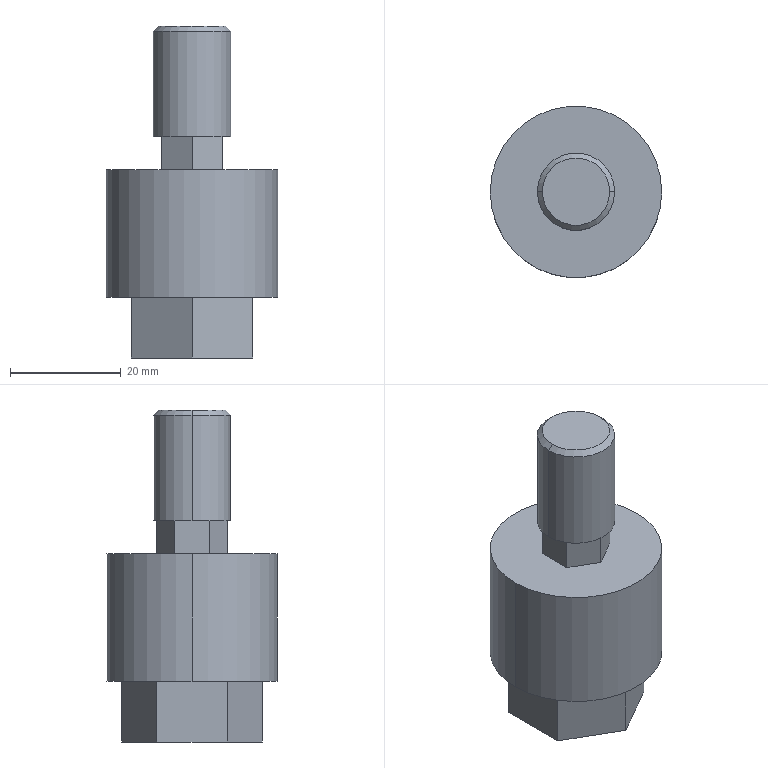Part | STEP file | JA40_14_150_JA40-14-150 | 1 solid | 28 faces | box 31 x 31 x 60 mm | volume 24083 mm3 | plane 18 | cylinder 6 | cone 4 | commonest cylinder face diameters 12.376 x2 14 x2 31 x2
STEP:
#1=CARTESIAN_POINT('',(-7.,0.,59.08));
#2=VERTEX_POINT('',#1);
#3=CARTESIAN_POINT('',(7.,0.,59.08));
#4=VERTEX_POINT('',#3);
#5=CARTESIAN_POINT('',(0.,0.,59.08));
#6=DIRECTION('',(0.,0.,-1.));
#7=DIRECTION('',(-1.,0.,0.));
#8=AXIS2_PLACEMENT_3D('',#5,#6,#7);
#9=CIRCLE('',#8,7.);
#10=EDGE_CURVE('',#2,#4,#9,.T.);
#11=ORIENTED_EDGE('',*,*,#10,.T.);
#12=CARTESIAN_POINT('',(7.,0.,40.));
#13=VERTEX_POINT('',#12);
#14=CARTESIAN_POINT('',(7.,0.,40.));
#15=DIRECTION('',(0.,0.,-1.));
#16=VECTOR('',#15,1000.);
#17=LINE('',#14,#16);
#18=EDGE_CURVE('',#4,#13,#17,.T.);
#19=ORIENTED_EDGE('',*,*,#18,.T.);
#20=CARTESIAN_POINT('',(-7.,0.,40.));
#21=VERTEX_POINT('',#20);
#22=CARTESIAN_POINT('',(0.,0.,40.));
#23=DIRECTION('',(0.,0.,-1.));
#24=DIRECTION('',(-1.,0.,0.));
#25=AXIS2_PLACEMENT_3D('',#22,#23,#24);
#26=CIRCLE('',#25,7.);
#27=EDGE_CURVE('',#21,#13,#26,.T.);
#28=ORIENTED_EDGE('',*,*,#27,.F.);
#29=CARTESIAN_POINT('',(-7.,0.,40.));
#30=DIRECTION('',(0.,0.,-1.));
#31=VECTOR('',#30,1000.);
#32=LINE('',#29,#31);
#33=EDGE_CURVE('',#2,#21,#32,.T.);
#34=ORIENTED_EDGE('',*,*,#33,.F.);
#35=EDGE_LOOP('',(#11,#19,#28,#34));
#36=FACE_OUTER_BOUND('',#35,.T.);
#37=CARTESIAN_POINT('',(0.,0.,40.));
#38=DIRECTION('',(0.,0.,-1.));
#39=DIRECTION('',(-1.,0.,0.));
#40=AXIS2_PLACEMENT_3D('',#37,#38,#39);
#41=CYLINDRICAL_SURFACE('',#40,7.);
#42=ADVANCED_FACE('',(#36),#41,.T.);
#43=CARTESIAN_POINT('',(-6.08,0.,60.));
#44=VERTEX_POINT('',#43);
#45=CARTESIAN_POINT('',(6.08,0.,60.));
#46=VERTEX_POINT('',#45);
#47=CARTESIAN_POINT('',(0.,0.,60.));
#48=DIRECTION('',(0.,0.,-1.));
#49=DIRECTION('',(-1.,0.,0.));
#50=AXIS2_PLACEMENT_3D('',#47,#48,#49);
#51=CIRCLE('',#50,6.08);
#52=EDGE_CURVE('',#44,#46,#51,.T.);
#53=ORIENTED_EDGE('',*,*,#52,.T.);
#54=CARTESIAN_POINT('',(7.,0.,59.08));
#55=DIRECTION('',(0.7071,0.,-0.7071));
#56=VECTOR('',#55,1000.);
#57=LINE('',#54,#56);
#58=EDGE_CURVE('',#46,#4,#57,.T.);
#59=ORIENTED_EDGE('',*,*,#58,.T.);
#60=ORIENTED_EDGE('',*,*,#10,.F.);
#61=CARTESIAN_POINT('',(-7.,0.,59.08));
#62=DIRECTION('',(-0.7071,0.,-0.7071));
#63=VECTOR('',#62,1000.);
#64=LINE('',#61,#63);
#65=EDGE_CURVE('',#44,#2,#64,.T.);
#66=ORIENTED_EDGE('',*,*,#65,.F.);
#67=EDGE_LOOP('',(#53,#59,#60,#66));
#68=FACE_OUTER_BOUND('',#67,.T.);
#69=CARTESIAN_POINT('',(0.,0.,59.08));
#70=DIRECTION('',(0.,0.,-1.));
#71=DIRECTION('',(-1.,0.,0.));
#72=AXIS2_PLACEMENT_3D('',#69,#70,#71);
#73=CONICAL_SURFACE('',#72,7.,0.7854);
#74=ADVANCED_FACE('',(#68),#73,.T.);
#75=CARTESIAN_POINT('',(6.188,0.,0.812));
#76=VERTEX_POINT('',#75);
#77=CARTESIAN_POINT('',(-6.188,0.,0.812));
#78=VERTEX_POINT('',#77);
#79=CARTESIAN_POINT('',(0.,0.,0.812));
#80=DIRECTION('',(0.,0.,-1.));
#81=DIRECTION('',(-1.,0.,0.));
#82=AXIS2_PLACEMENT_3D('',#79,#80,#81);
#83=CIRCLE('',#82,6.188);
#84=EDGE_CURVE('',#76,#78,#83,.T.);
#85=ORIENTED_EDGE('',*,*,#84,.F.);
#86=CARTESIAN_POINT('',(7.,0.,0.));
#87=VERTEX_POINT('',#86);
#88=CARTESIAN_POINT('',(6.188,0.,0.812));
#89=DIRECTION('',(0.7071,0.,-0.7071));
#90=VECTOR('',#89,1000.);
#91=LINE('',#88,#90);
#92=EDGE_CURVE('',#76,#87,#91,.T.);
#93=ORIENTED_EDGE('',*,*,#92,.T.);
#94=CARTESIAN_POINT('',(-7.,0.,0.));
#95=VERTEX_POINT('',#94);
#96=CARTESIAN_POINT('',(0.,0.,0.));
#97=DIRECTION('',(0.,0.,-1.));
#98=DIRECTION('',(-1.,0.,0.));
#99=AXIS2_PLACEMENT_3D('',#96,#97,#98);
#100=CIRCLE('',#99,7.);
#101=EDGE_CURVE('',#87,#95,#100,.T.);
#102=ORIENTED_EDGE('',*,*,#101,.T.);
#103=CARTESIAN_POINT('',(-6.188,0.,0.812));
#104=DIRECTION('',(-0.7071,0.,-0.7071));
#105=VECTOR('',#104,1000.);
#106=LINE('',#103,#105);
#107=EDGE_CURVE('',#78,#95,#106,.T.);
#108=ORIENTED_EDGE('',*,*,#107,.F.);
#109=EDGE_LOOP('',(#85,#93,#102,#108));
#110=FACE_OUTER_BOUND('',#109,.T.);
#111=CARTESIAN_POINT('',(0.,0.,0.812));
#112=DIRECTION('',(0.,0.,-1.));
#113=DIRECTION('',(-1.,0.,0.));
#114=AXIS2_PLACEMENT_3D('',#111,#112,#113);
#115=CONICAL_SURFACE('',#114,6.188,0.7854);
#116=ADVANCED_FACE('',(#110),#115,.F.);
#117=CARTESIAN_POINT('',(6.188,0.,13.));
#118=VERTEX_POINT('',#117);
#119=CARTESIAN_POINT('',(-6.188,0.,13.));
#120=VERTEX_POINT('',#119);
#121=CARTESIAN_POINT('',(0.,0.,13.));
#122=DIRECTION('',(0.,0.,-1.));
#123=DIRECTION('',(-1.,0.,0.));
#124=AXIS2_PLACEMENT_3D('',#121,#122,#123);
#125=CIRCLE('',#124,6.188);
#126=EDGE_CURVE('',#118,#120,#125,.T.);
#127=ORIENTED_EDGE('',*,*,#126,.F.);
#128=CARTESIAN_POINT('',(6.188,0.,0.));
#129=DIRECTION('',(0.,0.,-1.));
#130=VECTOR('',#129,1000.);
#131=LINE('',#128,#130);
#132=EDGE_CURVE('',#118,#76,#131,.T.);
#133=ORIENTED_EDGE('',*,*,#132,.T.);
#134=ORIENTED_EDGE('',*,*,#84,.T.);
#135=CARTESIAN_POINT('',(-6.188,0.,0.));
#136=DIRECTION('',(0.,0.,-1.));
#137=VECTOR('',#136,1000.);
#138=LINE('',#135,#137);
#139=EDGE_CURVE('',#120,#78,#138,.T.);
#140=ORIENTED_EDGE('',*,*,#139,.F.);
#141=EDGE_LOOP('',(#127,#133,#134,#140));
#142=FACE_OUTER_BOUND('',#141,.T.);
#143=CARTESIAN_POINT('',(0.,0.,0.));
#144=DIRECTION('',(0.,0.,-1.));
#145=DIRECTION('',(-1.,0.,0.));
#146=AXIS2_PLACEMENT_3D('',#143,#144,#145);
#147=CYLINDRICAL_SURFACE('',#146,6.188);
#148=ADVANCED_FACE('',(#142),#147,.F.);
#149=CARTESIAN_POINT('',(-15.5,0.,34.));
#150=VERTEX_POINT('',#149);
#151=CARTESIAN_POINT('',(15.5,0.,34.));
#152=VERTEX_POINT('',#151);
#153=CARTESIAN_POINT('',(0.,0.,34.));
#154=DIRECTION('',(0.,0.,-1.));
#155=DIRECTION('',(-1.,0.,0.));
#156=AXIS2_PLACEMENT_3D('',#153,#154,#155);
#157=CIRCLE('',#156,15.5);
#158=EDGE_CURVE('',#150,#152,#157,.T.);
#159=ORIENTED_EDGE('',*,*,#158,.T.);
#160=CARTESIAN_POINT('',(15.5,0.,11.));
#161=VERTEX_POINT('',#160);
#162=CARTESIAN_POINT('',(15.5,0.,0.));
#163=DIRECTION('',(0.,0.,-1.));
#164=VECTOR('',#163,1000.);
#165=LINE('',#162,#164);
#166=EDGE_CURVE('',#152,#161,#165,.T.);
#167=ORIENTED_EDGE('',*,*,#166,.T.);
#168=CARTESIAN_POINT('',(-15.5,0.,11.));
#169=VERTEX_POINT('',#168);
#170=CARTESIAN_POINT('',(0.,0.,11.));
#171=DIRECTION('',(0.,0.,-1.));
#172=DIRECTION('',(-1.,0.,0.));
#173=AXIS2_PLACEMENT_3D('',#170,#171,#172);
#174=CIRCLE('',#173,15.5);
#175=EDGE_CURVE('',#169,#161,#174,.T.);
#176=ORIENTED_EDGE('',*,*,#175,.F.);
#177=CARTESIAN_POINT('',(-15.5,0.,0.));
#178=DIRECTION('',(0.,0.,-1.));
#179=VECTOR('',#178,1000.);
#180=LINE('',#177,#179);
#181=EDGE_CURVE('',#150,#169,#180,.T.);
#182=ORIENTED_EDGE('',*,*,#181,.F.);
#183=EDGE_LOOP('',(#159,#167,#176,#182));
#184=FACE_OUTER_BOUND('',#183,.T.);
#185=CARTESIAN_POINT('',(0.,0.,0.));
#186=DIRECTION('',(0.,0.,-1.));
#187=DIRECTION('',(-1.,0.,0.));
#188=AXIS2_PLACEMENT_3D('',#185,#186,#187);
#189=CYLINDRICAL_SURFACE('',#188,15.5);
#190=ADVANCED_FACE('',(#184),#189,.T.);
#191=CARTESIAN_POINT('',(0.,6.351,40.));
#192=VERTEX_POINT('',#191);
#193=CARTESIAN_POINT('',(-5.5,3.175,40.));
#194=VERTEX_POINT('',#193);
#195=CARTESIAN_POINT('',(0.,6.351,40.));
#196=DIRECTION('',(-0.866,-0.5,0.));
#197=VECTOR('',#196,1000.);
#198=LINE('',#195,#197);
#199=EDGE_CURVE('',#192,#194,#198,.T.);
#200=ORIENTED_EDGE('',*,*,#199,.F.);
#201=CARTESIAN_POINT('',(0.,6.351,34.));
#202=VERTEX_POINT('',#201);
#203=CARTESIAN_POINT('',(0.,6.351,34.));
#204=DIRECTION('',(0.,0.,1.));
#205=VECTOR('',#204,1000.);
#206=LINE('',#203,#205);
#207=EDGE_CURVE('',#202,#192,#206,.T.);
#208=ORIENTED_EDGE('',*,*,#207,.F.);
#209=CARTESIAN_POINT('',(-5.5,3.175,34.));
#210=VERTEX_POINT('',#209);
#211=CARTESIAN_POINT('',(0.,6.351,34.));
#212=DIRECTION('',(-0.866,-0.5,0.));
#213=VECTOR('',#212,1000.);
#214=LINE('',#211,#213);
#215=EDGE_CURVE('',#202,#210,#214,.T.);
#216=ORIENTED_EDGE('',*,*,#215,.T.);
#217=CARTESIAN_POINT('',(-5.5,3.175,34.));
#218=DIRECTION('',(0.,0.,1.));
#219=VECTOR('',#218,1000.);
#220=LINE('',#217,#219);
#221=EDGE_CURVE('',#210,#194,#220,.T.);
#222=ORIENTED_EDGE('',*,*,#221,.T.);
#223=EDGE_LOOP('',(#200,#208,#216,#222));
#224=FACE_OUTER_BOUND('',#223,.T.);
#225=CARTESIAN_POINT('',(0.,6.351,34.));
#226=DIRECTION('',(-0.5,0.866,0.));
#227=DIRECTION('',(-0.866,-0.5,0.));
#228=AXIS2_PLACEMENT_3D('',#225,#226,#227);
#229=PLANE('',#228);
#230=ADVANCED_FACE('',(#224),#229,.T.);
#231=CARTESIAN_POINT('',(5.5,3.175,40.));
#232=VERTEX_POINT('',#231);
#233=CARTESIAN_POINT('',(5.5,3.175,40.));
#234=DIRECTION('',(-0.866,0.5,0.));
#235=VECTOR('',#234,1000.);
#236=LINE('',#233,#235);
#237=EDGE_CURVE('',#232,#192,#236,.T.);
#238=ORIENTED_EDGE('',*,*,#237,.F.);
#239=CARTESIAN_POINT('',(5.5,3.175,34.));
#240=VERTEX_POINT('',#239);
#241=CARTESIAN_POINT('',(5.5,3.175,34.));
#242=DIRECTION('',(0.,0.,1.));
#243=VECTOR('',#242,1000.);
#244=LINE('',#241,#243);
#245=EDGE_CURVE('',#240,#232,#244,.T.);
#246=ORIENTED_EDGE('',*,*,#245,.F.);
#247=CARTESIAN_POINT('',(5.5,3.175,34.));
#248=DIRECTION('',(-0.866,0.5,0.));
#249=VECTOR('',#248,1000.);
#250=LINE('',#247,#249);
#251=EDGE_CURVE('',#240,#202,#250,.T.);
#252=ORIENTED_EDGE('',*,*,#251,.T.);
#253=ORIENTED_EDGE('',*,*,#207,.T.);
#254=EDGE_LOOP('',(#238,#246,#252,#253));
#255=FACE_OUTER_BOUND('',#254,.T.);
#256=CARTESIAN_POINT('',(5.5,3.175,34.));
#257=DIRECTION('',(0.5,0.866,0.));
#258=DIRECTION('',(-0.866,0.5,0.));
#259=AXIS2_PLACEMENT_3D('',#256,#257,#258);
#260=PLANE('',#259);
#261=ADVANCED_FACE('',(#255),#260,.T.);
#262=CARTESIAN_POINT('',(5.5,-3.175,40.));
#263=VERTEX_POINT('',#262);
#264=CARTESIAN_POINT('',(5.5,-3.175,40.));
#265=DIRECTION('',(0.,1.,0.));
#266=VECTOR('',#265,1000.);
#267=LINE('',#264,#266);
#268=EDGE_CURVE('',#263,#232,#267,.T.);
#269=ORIENTED_EDGE('',*,*,#268,.F.);
#270=CARTESIAN_POINT('',(5.5,-3.175,34.));
#271=VERTEX_POINT('',#270);
#272=CARTESIAN_POINT('',(5.5,-3.175,34.));
#273=DIRECTION('',(0.,0.,1.));
#274=VECTOR('',#273,1000.);
#275=LINE('',#272,#274);
#276=EDGE_CURVE('',#271,#263,#275,.T.);
#277=ORIENTED_EDGE('',*,*,#276,.F.);
#278=CARTESIAN_POINT('',(5.5,-3.175,34.));
#279=DIRECTION('',(0.,1.,0.));
#280=VECTOR('',#279,1000.);
#281=LINE('',#278,#280);
#282=EDGE_CURVE('',#271,#240,#281,.T.);
#283=ORIENTED_EDGE('',*,*,#282,.T.);
#284=ORIENTED_EDGE('',*,*,#245,.T.);
#285=EDGE_LOOP('',(#269,#277,#283,#284));
#286=FACE_OUTER_BOUND('',#285,.T.);
#287=CARTESIAN_POINT('',(5.5,-3.175,34.));
#288=DIRECTION('',(1.,0.,0.));
#289=DIRECTION('',(0.,0.,-1.));
#290=AXIS2_PLACEMENT_3D('',#287,#288,#289);
#291=PLANE('',#290);
#292=ADVANCED_FACE('',(#286),#291,.T.);
#293=CARTESIAN_POINT('',(0.,-6.351,40.));
#294=VERTEX_POINT('',#293);
#295=CARTESIAN_POINT('',(0.,-6.351,40.));
#296=DIRECTION('',(0.866,0.5,0.));
#297=VECTOR('',#296,1000.);
#298=LINE('',#295,#297);
#299=EDGE_CURVE('',#294,#263,#298,.T.);
#300=ORIENTED_EDGE('',*,*,#299,.F.);
#301=CARTESIAN_POINT('',(0.,-6.351,34.));
#302=VERTEX_POINT('',#301);
#303=CARTESIAN_POINT('',(0.,-6.351,34.));
#304=DIRECTION('',(0.,0.,1.));
#305=VECTOR('',#304,1000.);
#306=LINE('',#303,#305);
#307=EDGE_CURVE('',#302,#294,#306,.T.);
#308=ORIENTED_EDGE('',*,*,#307,.F.);
#309=CARTESIAN_POINT('',(0.,-6.351,34.));
#310=DIRECTION('',(0.866,0.5,0.));
#311=VECTOR('',#310,1000.);
#312=LINE('',#309,#311);
#313=EDGE_CURVE('',#302,#271,#312,.T.);
#314=ORIENTED_EDGE('',*,*,#313,.T.);
#315=ORIENTED_EDGE('',*,*,#276,.T.);
#316=EDGE_LOOP('',(#300,#308,#314,#315));
#317=FACE_OUTER_BOUND('',#316,.T.);
#318=CARTESIAN_POINT('',(0.,-6.351,34.));
#319=DIRECTION('',(0.5,-0.866,0.));
#320=DIRECTION('',(0.866,0.5,0.));
#321=AXIS2_PLACEMENT_3D('',#318,#319,#320);
#322=PLANE('',#321);
#323=ADVANCED_FACE('',(#317),#322,.T.);
#324=CARTESIAN_POINT('',(-5.5,-3.175,40.));
#325=VERTEX_POINT('',#324);
#326=CARTESIAN_POINT('',(-5.5,-3.175,40.));
#327=DIRECTION('',(0.866,-0.5,0.));
#328=VECTOR('',#327,1000.);
#329=LINE('',#326,#328);
#330=EDGE_CURVE('',#325,#294,#329,.T.);
#331=ORIENTED_EDGE('',*,*,#330,.F.);
#332=CARTESIAN_POINT('',(-5.5,-3.175,34.));
#333=VERTEX_POINT('',#332);
#334=CARTESIAN_POINT('',(-5.5,-3.175,34.));
#335=DIRECTION('',(0.,0.,1.));
#336=VECTOR('',#335,1000.);
#337=LINE('',#334,#336);
#338=EDGE_CURVE('',#333,#325,#337,.T.);
#339=ORIENTED_EDGE('',*,*,#338,.F.);
#340=CARTESIAN_POINT('',(-5.5,-3.175,34.));
#341=DIRECTION('',(0.866,-0.5,0.));
#342=VECTOR('',#341,1000.);
#343=LINE('',#340,#342);
#344=EDGE_CURVE('',#333,#302,#343,.T.);
#345=ORIENTED_EDGE('',*,*,#344,.T.);
#346=ORIENTED_EDGE('',*,*,#307,.T.);
#347=EDGE_LOOP('',(#331,#339,#345,#346));
#348=FACE_OUTER_BOUND('',#347,.T.);
#349=CARTESIAN_POINT('',(-5.5,-3.175,34.));
#350=DIRECTION('',(-0.5,-0.866,0.));
#351=DIRECTION('',(0.866,-0.5,0.));
#352=AXIS2_PLACEMENT_3D('',#349,#350,#351);
#353=PLANE('',#352);
#354=ADVANCED_FACE('',(#348),#353,.T.);
#355=CARTESIAN_POINT('',(-5.5,3.175,40.));
#356=DIRECTION('',(0.,-1.,0.));
#357=VECTOR('',#356,1000.);
#358=LINE('',#355,#357);
#359=EDGE_CURVE('',#194,#325,#358,.T.);
#360=ORIENTED_EDGE('',*,*,#359,.F.);
#361=ORIENTED_EDGE('',*,*,#221,.F.);
#362=CARTESIAN_POINT('',(-5.5,3.175,34.));
#363=DIRECTION('',(0.,-1.,0.));
#364=VECTOR('',#363,1000.);
#365=LINE('',#362,#364);
#366=EDGE_CURVE('',#210,#333,#365,.T.);
#367=ORIENTED_EDGE('',*,*,#366,.T.);
#368=ORIENTED_EDGE('',*,*,#338,.T.);
#369=EDGE_LOOP('',(#360,#361,#367,#368));
#370=FACE_OUTER_BOUND('',#369,.T.);
#371=CARTESIAN_POINT('',(-5.5,3.175,34.));
#372=DIRECTION('',(-1.,0.,0.));
#373=DIRECTION('',(0.,0.,1.));
#374=AXIS2_PLACEMENT_3D('',#371,#372,#373);
#375=PLANE('',#374);
#376=ADVANCED_FACE('',(#370),#375,.T.);
#377=ORIENTED_EDGE('',*,*,#366,.F.);
#378=ORIENTED_EDGE('',*,*,#215,.F.);
#379=ORIENTED_EDGE('',*,*,#251,.F.);
#380=ORIENTED_EDGE('',*,*,#282,.F.);
#381=ORIENTED_EDGE('',*,*,#313,.F.);
#382=ORIENTED_EDGE('',*,*,#344,.F.);
#383=EDGE_LOOP('',(#377,#378,#379,#380,#381,#382));
#384=FACE_BOUND('',#383,.T.);
#385=ORIENTED_EDGE('',*,*,#158,.F.);
#386=CARTESIAN_POINT('',(0.,0.,34.));
#387=DIRECTION('',(0.,0.,-1.));
#388=DIRECTION('',(-1.,0.,0.));
#389=AXIS2_PLACEMENT_3D('',#386,#387,#388);
#390=CIRCLE('',#389,15.5);
#391=EDGE_CURVE('',#152,#150,#390,.T.);
#392=ORIENTED_EDGE('',*,*,#391,.F.);
#393=EDGE_LOOP('',(#385,#392));
#394=FACE_OUTER_BOUND('',#393,.T.);
#395=CARTESIAN_POINT('',(0.,0.,34.));
#396=DIRECTION('',(0.,0.,1.));
#397=DIRECTION('',(1.,0.,0.));
#398=AXIS2_PLACEMENT_3D('',#395,#396,#397);
#399=PLANE('',#398);
#400=ADVANCED_FACE('',(#384,#394),#399,.T.);
#401=ORIENTED_EDGE('',*,*,#166,.F.);
#402=ORIENTED_EDGE('',*,*,#391,.T.);
#403=ORIENTED_EDGE('',*,*,#181,.T.);
#404=CARTESIAN_POINT('',(0.,0.,11.));
#405=DIRECTION('',(0.,0.,-1.));
#406=DIRECTION('',(-1.,0.,0.));
#407=AXIS2_PLACEMENT_3D('',#404,#405,#406);
#408=CIRCLE('',#407,15.5);
#409=EDGE_CURVE('',#161,#169,#408,.T.);
#410=ORIENTED_EDGE('',*,*,#409,.F.);
#411=EDGE_LOOP('',(#401,#402,#403,#410));
#412=FACE_OUTER_BOUND('',#411,.T.);
#413=CARTESIAN_POINT('',(0.,0.,0.));
#414=DIRECTION('',(0.,0.,-1.));
#415=DIRECTION('',(-1.,0.,0.));
#416=AXIS2_PLACEMENT_3D('',#413,#414,#415);
#417=CYLINDRICAL_SURFACE('',#416,15.5);
#418=ADVANCED_FACE('',(#412),#417,.T.);
#419=ORIENTED_EDGE('',*,*,#175,.T.);
#420=ORIENTED_EDGE('',*,*,#409,.T.);
#421=EDGE_LOOP('',(#419,#420));
#422=FACE_OUTER_BOUND('',#421,.T.);
#423=CARTESIAN_POINT('',(-11.,6.351,11.));
#424=VERTEX_POINT('',#423);
#425=CARTESIAN_POINT('',(-11.,-6.351,11.));
#426=VERTEX_POINT('',#425);
#427=CARTESIAN_POINT('',(-11.,6.351,11.));
#428=DIRECTION('',(0.,-1.,0.));
#429=VECTOR('',#428,1000.);
#430=LINE('',#427,#429);
#431=EDGE_CURVE('',#424,#426,#430,.T.);
#432=ORIENTED_EDGE('',*,*,#431,.T.);
#433=CARTESIAN_POINT('',(0.,-12.702,11.));
#434=VERTEX_POINT('',#433);
#435=CARTESIAN_POINT('',(-11.,-6.351,11.));
#436=DIRECTION('',(0.866,-0.5,0.));
#437=VECTOR('',#436,1000.);
#438=LINE('',#435,#437);
#439=EDGE_CURVE('',#426,#434,#438,.T.);
#440=ORIENTED_EDGE('',*,*,#439,.T.);
#441=CARTESIAN_POINT('',(11.,-6.351,11.));
#442=VERTEX_POINT('',#441);
#443=CARTESIAN_POINT('',(0.,-12.702,11.));
#444=DIRECTION('',(0.866,0.5,0.));
#445=VECTOR('',#444,1000.);
#446=LINE('',#443,#445);
#447=EDGE_CURVE('',#434,#442,#446,.T.);
#448=ORIENTED_EDGE('',*,*,#447,.T.);
#449=CARTESIAN_POINT('',(11.,6.351,11.));
#450=VERTEX_POINT('',#449);
#451=CARTESIAN_POINT('',(11.,-6.351,11.));
#452=DIRECTION('',(0.,1.,0.));
#453=VECTOR('',#452,1000.);
#454=LINE('',#451,#453);
#455=EDGE_CURVE('',#442,#450,#454,.T.);
#456=ORIENTED_EDGE('',*,*,#455,.T.);
#457=CARTESIAN_POINT('',(0.,12.702,11.));
#458=VERTEX_POINT('',#457);
#459=CARTESIAN_POINT('',(11.,6.351,11.));
#460=DIRECTION('',(-0.866,0.5,0.));
#461=VECTOR('',#460,1000.);
#462=LINE('',#459,#461);
#463=EDGE_CURVE('',#450,#458,#462,.T.);
#464=ORIENTED_EDGE('',*,*,#463,.T.);
#465=CARTESIAN_POINT('',(0.,12.702,11.));
#466=DIRECTION('',(-0.866,-0.5,0.));
#467=VECTOR('',#466,1000.);
#468=LINE('',#465,#467);
#469=EDGE_CURVE('',#458,#424,#468,.T.);
#470=ORIENTED_EDGE('',*,*,#469,.T.);
#471=EDGE_LOOP('',(#432,#440,#448,#456,#464,#470));
#472=FACE_BOUND('',#471,.T.);
#473=CARTESIAN_POINT('',(0.,15.5,11.));
#474=DIRECTION('',(0.,0.,-1.));
#475=DIRECTION('',(-1.,0.,0.));
#476=AXIS2_PLACEMENT_3D('',#473,#474,#475);
#477=PLANE('',#476);
#478=ADVANCED_FACE('',(#422,#472),#477,.T.);
#479=CARTESIAN_POINT('',(0.,12.702,0.));
#480=VERTEX_POINT('',#479);
#481=CARTESIAN_POINT('',(-11.,6.351,0.));
#482=VERTEX_POINT('',#481);
#483=CARTESIAN_POINT('',(0.,12.702,0.));
#484=DIRECTION('',(-0.866,-0.5,0.));
#485=VECTOR('',#484,1000.);
#486=LINE('',#483,#485);
#487=EDGE_CURVE('',#480,#482,#486,.T.);
#488=ORIENTED_EDGE('',*,*,#487,.T.);
#489=CARTESIAN_POINT('',(-11.,6.351,11.));
#490=DIRECTION('',(0.,0.,-1.));
#491=VECTOR('',#490,1000.);
#492=LINE('',#489,#491);
#493=EDGE_CURVE('',#424,#482,#492,.T.);
#494=ORIENTED_EDGE('',*,*,#493,.F.);
#495=ORIENTED_EDGE('',*,*,#469,.F.);
#496=CARTESIAN_POINT('',(0.,12.702,11.));
#497=DIRECTION('',(0.,0.,-1.));
#498=VECTOR('',#497,1000.);
#499=LINE('',#496,#498);
#500=EDGE_CURVE('',#458,#480,#499,.T.);
#501=ORIENTED_EDGE('',*,*,#500,.T.);
#502=EDGE_LOOP('',(#488,#494,#495,#501));
#503=FACE_OUTER_BOUND('',#502,.T.);
#504=CARTESIAN_POINT('',(0.,12.702,11.));
#505=DIRECTION('',(0.5,-0.866,0.));
#506=DIRECTION('',(0.866,0.5,0.));
#507=AXIS2_PLACEMENT_3D('',#504,#505,#506);
#508=PLANE('',#507);
#509=ADVANCED_FACE('',(#503),#508,.F.);
#510=CARTESIAN_POINT('',(-11.,-6.351,0.));
#511=VERTEX_POINT('',#510);
#512=CARTESIAN_POINT('',(-11.,6.351,0.));
#513=DIRECTION('',(0.,-1.,0.));
#514=VECTOR('',#513,1000.);
#515=LINE('',#512,#514);
#516=EDGE_CURVE('',#482,#511,#515,.T.);
#517=ORIENTED_EDGE('',*,*,#516,.T.);
#518=CARTESIAN_POINT('',(-11.,-6.351,11.));
#519=DIRECTION('',(0.,0.,-1.));
#520=VECTOR('',#519,1000.);
#521=LINE('',#518,#520);
#522=EDGE_CURVE('',#426,#511,#521,.T.);
#523=ORIENTED_EDGE('',*,*,#522,.F.);
#524=ORIENTED_EDGE('',*,*,#431,.F.);
#525=ORIENTED_EDGE('',*,*,#493,.T.);
#526=EDGE_LOOP('',(#517,#523,#524,#525));
#527=FACE_OUTER_BOUND('',#526,.T.);
#528=CARTESIAN_POINT('',(-11.,6.351,11.));
#529=DIRECTION('',(1.,0.,0.));
#530=DIRECTION('',(0.,0.,-1.));
#531=AXIS2_PLACEMENT_3D('',#528,#529,#530);
#532=PLANE('',#531);
#533=ADVANCED_FACE('',(#527),#532,.F.);
#534=CARTESIAN_POINT('',(0.,-12.702,0.));
#535=VERTEX_POINT('',#534);
#536=CARTESIAN_POINT('',(-11.,-6.351,0.));
#537=DIRECTION('',(0.866,-0.5,0.));
#538=VECTOR('',#537,1000.);
#539=LINE('',#536,#538);
#540=EDGE_CURVE('',#511,#535,#539,.T.);
#541=ORIENTED_EDGE('',*,*,#540,.T.);
#542=CARTESIAN_POINT('',(0.,-12.702,11.));
#543=DIRECTION('',(0.,0.,-1.));
#544=VECTOR('',#543,1000.);
#545=LINE('',#542,#544);
#546=EDGE_CURVE('',#434,#535,#545,.T.);
#547=ORIENTED_EDGE('',*,*,#546,.F.);
#548=ORIENTED_EDGE('',*,*,#439,.F.);
#549=ORIENTED_EDGE('',*,*,#522,.T.);
#550=EDGE_LOOP('',(#541,#547,#548,#549));
#551=FACE_OUTER_BOUND('',#550,.T.);
#552=CARTESIAN_POINT('',(-11.,-6.351,11.));
#553=DIRECTION('',(0.5,0.866,0.));
#554=DIRECTION('',(-0.866,0.5,0.));
#555=AXIS2_PLACEMENT_3D('',#552,#553,#554);
#556=PLANE('',#555);
#557=ADVANCED_FACE('',(#551),#556,.F.);
#558=CARTESIAN_POINT('',(11.,-6.351,0.));
#559=VERTEX_POINT('',#558);
#560=CARTESIAN_POINT('',(0.,-12.702,0.));
#561=DIRECTION('',(0.866,0.5,0.));
#562=VECTOR('',#561,1000.);
#563=LINE('',#560,#562);
#564=EDGE_CURVE('',#535,#559,#563,.T.);
#565=ORIENTED_EDGE('',*,*,#564,.T.);
#566=CARTESIAN_POINT('',(11.,-6.351,11.));
#567=DIRECTION('',(0.,0.,-1.));
#568=VECTOR('',#567,1000.);
#569=LINE('',#566,#568);
#570=EDGE_CURVE('',#442,#559,#569,.T.);
#571=ORIENTED_EDGE('',*,*,#570,.F.);
#572=ORIENTED_EDGE('',*,*,#447,.F.);
#573=ORIENTED_EDGE('',*,*,#546,.T.);
#574=EDGE_LOOP('',(#565,#571,#572,#573));
#575=FACE_OUTER_BOUND('',#574,.T.);
#576=CARTESIAN_POINT('',(0.,-12.702,11.));
#577=DIRECTION('',(-0.5,0.866,0.));
#578=DIRECTION('',(-0.866,-0.5,0.));
#579=AXIS2_PLACEMENT_3D('',#576,#577,#578);
#580=PLANE('',#579);
#581=ADVANCED_FACE('',(#575),#580,.F.);
#582=CARTESIAN_POINT('',(11.,6.351,0.));
#583=VERTEX_POINT('',#582);
#584=CARTESIAN_POINT('',(11.,-6.351,0.));
#585=DIRECTION('',(0.,1.,0.));
#586=VECTOR('',#585,1000.);
#587=LINE('',#584,#586);
#588=EDGE_CURVE('',#559,#583,#587,.T.);
#589=ORIENTED_EDGE('',*,*,#588,.T.);
#590=CARTESIAN_POINT('',(11.,6.351,11.));
#591=DIRECTION('',(0.,0.,-1.));
#592=VECTOR('',#591,1000.);
#593=LINE('',#590,#592);
#594=EDGE_CURVE('',#450,#583,#593,.T.);
#595=ORIENTED_EDGE('',*,*,#594,.F.);
#596=ORIENTED_EDGE('',*,*,#455,.F.);
#597=ORIENTED_EDGE('',*,*,#570,.T.);
#598=EDGE_LOOP('',(#589,#595,#596,#597));
#599=FACE_OUTER_BOUND('',#598,.T.);
#600=CARTESIAN_POINT('',(11.,-6.351,11.));
#601=DIRECTION('',(-1.,0.,0.));
#602=DIRECTION('',(0.,0.,1.));
#603=AXIS2_PLACEMENT_3D('',#600,#601,#602);
#604=PLANE('',#603);
#605=ADVANCED_FACE('',(#599),#604,.F.);
#606=CARTESIAN_POINT('',(11.,6.351,0.));
#607=DIRECTION('',(-0.866,0.5,0.));
#608=VECTOR('',#607,1000.);
#609=LINE('',#606,#608);
#610=EDGE_CURVE('',#583,#480,#609,.T.);
#611=ORIENTED_EDGE('',*,*,#610,.T.);
#612=ORIENTED_EDGE('',*,*,#500,.F.);
#613=ORIENTED_EDGE('',*,*,#463,.F.);
#614=ORIENTED_EDGE('',*,*,#594,.T.);
#615=EDGE_LOOP('',(#611,#612,#613,#614));
#616=FACE_OUTER_BOUND('',#615,.T.);
#617=CARTESIAN_POINT('',(11.,6.351,11.));
#618=DIRECTION('',(-0.5,-0.866,0.));
#619=DIRECTION('',(0.866,-0.5,0.));
#620=AXIS2_PLACEMENT_3D('',#617,#618,#619);
#621=PLANE('',#620);
#622=ADVANCED_FACE('',(#616),#621,.F.);
#623=CARTESIAN_POINT('',(0.,0.,13.));
#624=DIRECTION('',(0.,0.,-1.));
#625=DIRECTION('',(-1.,0.,0.));
#626=AXIS2_PLACEMENT_3D('',#623,#624,#625);
#627=CIRCLE('',#626,6.188);
#628=EDGE_CURVE('',#120,#118,#627,.T.);
#629=ORIENTED_EDGE('',*,*,#628,.T.);
#630=ORIENTED_EDGE('',*,*,#126,.T.);
#631=EDGE_LOOP('',(#629,#630));
#632=FACE_OUTER_BOUND('',#631,.T.);
#633=CARTESIAN_POINT('',(0.,6.188,13.));
#634=DIRECTION('',(0.,0.,-1.));
#635=DIRECTION('',(-1.,0.,0.));
#636=AXIS2_PLACEMENT_3D('',#633,#634,#635);
#637=PLANE('',#636);
#638=ADVANCED_FACE('',(#632),#637,.T.);
#639=ORIENTED_EDGE('',*,*,#132,.F.);
#640=ORIENTED_EDGE('',*,*,#628,.F.);
#641=ORIENTED_EDGE('',*,*,#139,.T.);
#642=CARTESIAN_POINT('',(0.,0.,0.812));
#643=DIRECTION('',(0.,0.,-1.));
#644=DIRECTION('',(-1.,0.,0.));
#645=AXIS2_PLACEMENT_3D('',#642,#643,#644);
#646=CIRCLE('',#645,6.188);
#647=EDGE_CURVE('',#78,#76,#646,.T.);
#648=ORIENTED_EDGE('',*,*,#647,.T.);
#649=EDGE_LOOP('',(#639,#640,#641,#648));
#650=FACE_OUTER_BOUND('',#649,.T.);
#651=CARTESIAN_POINT('',(0.,0.,0.));
#652=DIRECTION('',(0.,0.,-1.));
#653=DIRECTION('',(-1.,0.,0.));
#654=AXIS2_PLACEMENT_3D('',#651,#652,#653);
#655=CYLINDRICAL_SURFACE('',#654,6.188);
#656=ADVANCED_FACE('',(#650),#655,.F.);
#657=ORIENTED_EDGE('',*,*,#92,.F.);
#658=ORIENTED_EDGE('',*,*,#647,.F.);
#659=ORIENTED_EDGE('',*,*,#107,.T.);
#660=CARTESIAN_POINT('',(0.,0.,0.));
#661=DIRECTION('',(0.,0.,-1.));
#662=DIRECTION('',(-1.,0.,0.));
#663=AXIS2_PLACEMENT_3D('',#660,#661,#662);
#664=CIRCLE('',#663,7.);
#665=EDGE_CURVE('',#95,#87,#664,.T.);
#666=ORIENTED_EDGE('',*,*,#665,.T.);
#667=EDGE_LOOP('',(#657,#658,#659,#666));
#668=FACE_OUTER_BOUND('',#667,.T.);
#669=CARTESIAN_POINT('',(0.,0.,0.812));
#670=DIRECTION('',(0.,0.,-1.));
#671=DIRECTION('',(-1.,0.,0.));
#672=AXIS2_PLACEMENT_3D('',#669,#670,#671);
#673=CONICAL_SURFACE('',#672,6.188,0.7854);
#674=ADVANCED_FACE('',(#668),#673,.F.);
#675=ORIENTED_EDGE('',*,*,#487,.F.);
#676=ORIENTED_EDGE('',*,*,#610,.F.);
#677=ORIENTED_EDGE('',*,*,#588,.F.);
#678=ORIENTED_EDGE('',*,*,#564,.F.);
#679=ORIENTED_EDGE('',*,*,#540,.F.);
#680=ORIENTED_EDGE('',*,*,#516,.F.);
#681=EDGE_LOOP('',(#675,#676,#677,#678,#679,#680));
#682=FACE_OUTER_BOUND('',#681,.T.);
#683=ORIENTED_EDGE('',*,*,#665,.F.);
#684=ORIENTED_EDGE('',*,*,#101,.F.);
#685=EDGE_LOOP('',(#683,#684));
#686=FACE_BOUND('',#685,.T.);
#687=CARTESIAN_POINT('',(0.,13.2,0.));
#688=DIRECTION('',(0.,0.,-1.));
#689=DIRECTION('',(-1.,0.,0.));
#690=AXIS2_PLACEMENT_3D('',#687,#688,#689);
#691=PLANE('',#690);
#692=ADVANCED_FACE('',(#682,#686),#691,.T.);
#693=ORIENTED_EDGE('',*,*,#52,.F.);
#694=CARTESIAN_POINT('',(0.,0.,60.));
#695=DIRECTION('',(0.,0.,-1.));
#696=DIRECTION('',(-1.,0.,0.));
#697=AXIS2_PLACEMENT_3D('',#694,#695,#696);
#698=CIRCLE('',#697,6.08);
#699=EDGE_CURVE('',#46,#44,#698,.T.);
#700=ORIENTED_EDGE('',*,*,#699,.F.);
#701=EDGE_LOOP('',(#693,#700));
#702=FACE_OUTER_BOUND('',#701,.T.);
#703=CARTESIAN_POINT('',(0.,0.,60.));
#704=DIRECTION('',(0.,0.,1.));
#705=DIRECTION('',(1.,0.,0.));
#706=AXIS2_PLACEMENT_3D('',#703,#704,#705);
#707=PLANE('',#706);
#708=ADVANCED_FACE('',(#702),#707,.T.);
#709=ORIENTED_EDGE('',*,*,#58,.F.);
#710=ORIENTED_EDGE('',*,*,#699,.T.);
#711=ORIENTED_EDGE('',*,*,#65,.T.);
#712=CARTESIAN_POINT('',(0.,0.,59.08));
#713=DIRECTION('',(0.,0.,-1.));
#714=DIRECTION('',(-1.,0.,0.));
#715=AXIS2_PLACEMENT_3D('',#712,#713,#714);
#716=CIRCLE('',#715,7.);
#717=EDGE_CURVE('',#4,#2,#716,.T.);
#718=ORIENTED_EDGE('',*,*,#717,.F.);
#719=EDGE_LOOP('',(#709,#710,#711,#718));
#720=FACE_OUTER_BOUND('',#719,.T.);
#721=CARTESIAN_POINT('',(0.,0.,59.08));
#722=DIRECTION('',(0.,0.,-1.));
#723=DIRECTION('',(-1.,0.,0.));
#724=AXIS2_PLACEMENT_3D('',#721,#722,#723);
#725=CONICAL_SURFACE('',#724,7.,0.7854);
#726=ADVANCED_FACE('',(#720),#725,.T.);
#727=ORIENTED_EDGE('',*,*,#18,.F.);
#728=ORIENTED_EDGE('',*,*,#717,.T.);
#729=ORIENTED_EDGE('',*,*,#33,.T.);
#730=CARTESIAN_POINT('',(0.,0.,40.));
#731=DIRECTION('',(0.,0.,-1.));
#732=DIRECTION('',(-1.,0.,0.));
#733=AXIS2_PLACEMENT_3D('',#730,#731,#732);
#734=CIRCLE('',#733,7.);
#735=EDGE_CURVE('',#13,#21,#734,.T.);
#736=ORIENTED_EDGE('',*,*,#735,.F.);
#737=EDGE_LOOP('',(#727,#728,#729,#736));
#738=FACE_OUTER_BOUND('',#737,.T.);
#739=CARTESIAN_POINT('',(0.,0.,40.));
#740=DIRECTION('',(0.,0.,-1.));
#741=DIRECTION('',(-1.,0.,0.));
#742=AXIS2_PLACEMENT_3D('',#739,#740,#741);
#743=CYLINDRICAL_SURFACE('',#742,7.);
#744=ADVANCED_FACE('',(#738),#743,.T.);
#745=ORIENTED_EDGE('',*,*,#237,.T.);
#746=ORIENTED_EDGE('',*,*,#199,.T.);
#747=ORIENTED_EDGE('',*,*,#359,.T.);
#748=ORIENTED_EDGE('',*,*,#330,.T.);
#749=ORIENTED_EDGE('',*,*,#299,.T.);
#750=ORIENTED_EDGE('',*,*,#268,.T.);
#751=EDGE_LOOP('',(#745,#746,#747,#748,#749,#750));
#752=FACE_BOUND('',#751,.T.);
#753=ORIENTED_EDGE('',*,*,#27,.T.);
#754=ORIENTED_EDGE('',*,*,#735,.T.);
#755=EDGE_LOOP('',(#753,#754));
#756=FACE_OUTER_BOUND('',#755,.T.);
#757=CARTESIAN_POINT('',(0.,7.,40.));
#758=DIRECTION('',(0.,0.,-1.));
#759=DIRECTION('',(-1.,0.,0.));
#760=AXIS2_PLACEMENT_3D('',#757,#758,#759);
#761=PLANE('',#760);
#762=ADVANCED_FACE('',(#752,#756),#761,.T.);
#763=CLOSED_SHELL('',(#42,#74,#116,#148,#190,#230,#261,#292,#323,#354,#376,#400,#418,#478,#509,#533,#557,#581,#605,#622,#638,#656,#674,#692,#708,#726,#744,#762));
#764=MANIFOLD_SOLID_BREP('',#763);
#765=CARTESIAN_POINT('',(0.,0.,0.));
#766=DIRECTION('',(0.,0.,1.));
#767=DIRECTION('',(1.,0.,0.));
#768=AXIS2_PLACEMENT_3D('',#765,#766,#767);
#769=(LENGTH_UNIT()NAMED_UNIT(*)SI_UNIT(.MILLI.,.METRE.));
#770=UNCERTAINTY_MEASURE_WITH_UNIT(LENGTH_MEASURE(0.00001),#769,'','');
#771=(NAMED_UNIT(*)PLANE_ANGLE_UNIT()SI_UNIT($,.RADIAN.));
#772=(NAMED_UNIT(*)SI_UNIT($,.STERADIAN.)SOLID_ANGLE_UNIT());
#773=(GEOMETRIC_REPRESENTATION_CONTEXT(3)GLOBAL_UNCERTAINTY_ASSIGNED_CONTEXT((#770))GLOBAL_UNIT_ASSIGNED_CONTEXT((#769,#771,#772))REPRESENTATION_CONTEXT('',''));
#774=ADVANCED_BREP_SHAPE_REPRESENTATION('',(#764,#768),#773);